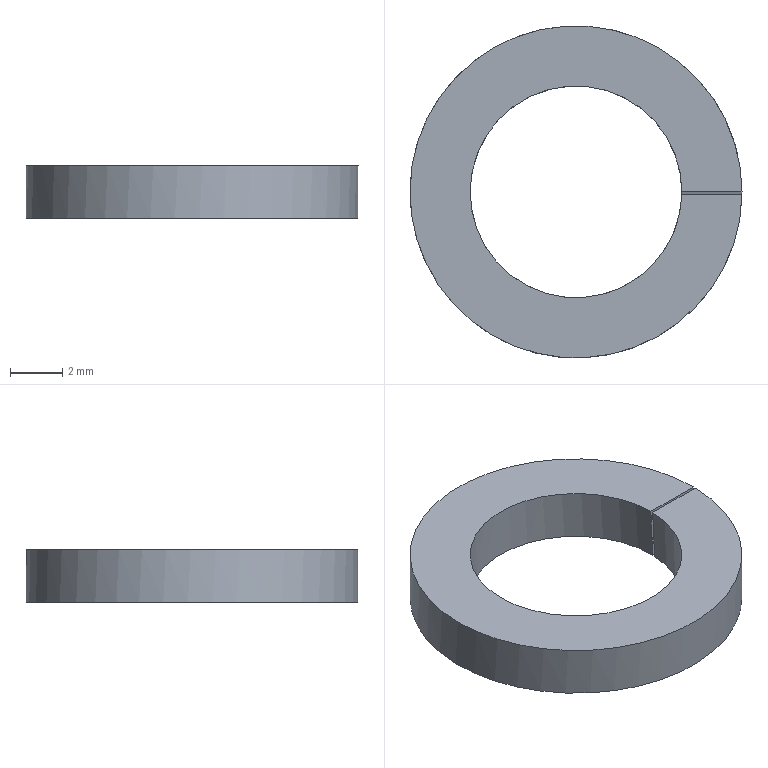Part | STEP file | SOLID | 1 solid | 6 faces | box 12.7 x 12.7 x 2 mm | volume 149.833 mm3 | plane 4 | cylinder 2 | commonest cylinder face diameters 8.1 x1 12.7 x1
STEP:
#1=CARTESIAN_POINT('',(0.,0.,0.));
#2=DIRECTION('',(0.,0.,1.));
#3=DIRECTION('',(1.,0.,0.));
#4=AXIS2_PLACEMENT_3D('',#1,#2,#3);
#5=CARTESIAN_POINT('',(6.349,-0.1,0.));
#6=VERTEX_POINT('',#5);
#7=CARTESIAN_POINT('',(6.347,-0.2048,-2.));
#8=VERTEX_POINT('',#7);
#9=CARTESIAN_POINT('',(0.,0.,1.908));
#10=DIRECTION('',(0.,0.9986,-0.05234));
#11=DIRECTION('',(0.,0.05234,0.9986));
#12=AXIS2_PLACEMENT_3D('',#9,#10,#11);
#13=ELLIPSE('',#12,121.331,6.35);
#14=CARTESIAN_POINT('',(0.,0.,-1.2));
#15=DIRECTION('',(0.,0.,1.));
#16=DIRECTION('',(1.,0.,0.));
#17=AXIS2_PLACEMENT_3D('',#14,#15,#16);
#18=CYLINDRICAL_SURFACE('',#17,6.35);
#19=CARTESIAN_POINT('',(6.267,1.2));
#20=CARTESIAN_POINT('',(6.267,1.17));
#21=CARTESIAN_POINT('',(6.267,1.109));
#22=CARTESIAN_POINT('',(6.266,1.018));
#23=CARTESIAN_POINT('',(6.265,0.9272));
#24=CARTESIAN_POINT('',(6.264,0.8363));
#25=CARTESIAN_POINT('',(6.264,0.7454));
#26=CARTESIAN_POINT('',(6.263,0.6545));
#27=CARTESIAN_POINT('',(6.262,0.5636));
#28=CARTESIAN_POINT('',(6.261,0.4726));
#29=CARTESIAN_POINT('',(6.261,0.3817));
#30=CARTESIAN_POINT('',(6.26,0.2908));
#31=CARTESIAN_POINT('',(6.259,0.1999));
#32=CARTESIAN_POINT('',(6.258,0.109));
#33=CARTESIAN_POINT('',(6.258,0.01808));
#34=CARTESIAN_POINT('',(6.257,-0.07282));
#35=CARTESIAN_POINT('',(6.256,-0.1637));
#36=CARTESIAN_POINT('',(6.255,-0.2546));
#37=CARTESIAN_POINT('',(6.255,-0.3455));
#38=CARTESIAN_POINT('',(6.254,-0.4364));
#39=CARTESIAN_POINT('',(6.253,-0.5273));
#40=CARTESIAN_POINT('',(6.252,-0.6182));
#41=CARTESIAN_POINT('',(6.252,-0.7091));
#42=CARTESIAN_POINT('',(6.251,-0.7697));
#43=CARTESIAN_POINT('',(6.251,-0.8));
#44=B_SPLINE_CURVE_WITH_KNOTS('',3,(#19,#20,#21,#22,#23,#24,#25,#26,#27,#28,#29,#30,#31,#32,#33,#34,#35,#36,#37,#38,#39,#40,#41,#42,#43),.UNSPECIFIED.,.F.,.F.,(4,1,1,1,1,1,1,1,1,1,1,1,1,1,1,1,1,1,1,1,1,1,4),(1.587,1.587,1.588,1.589,1.59,1.59,1.591,1.592,1.593,1.593,1.594,1.595,1.596,1.596,1.597,1.598,1.599,1.599,1.6,1.601,1.602,1.602,1.603),.QUASI_UNIFORM_KNOTS.);
#45=(GEOMETRIC_REPRESENTATION_CONTEXT(2)PARAMETRIC_REPRESENTATION_CONTEXT()REPRESENTATION_CONTEXT('',''));
#46=DEFINITIONAL_REPRESENTATION('',(#44),#45);
#47=PCURVE('',#18,#46);
#48=CARTESIAN_POINT('',(6.653,-0.1,0.));
#49=DIRECTION('',(0.,-0.9986,0.05234));
#50=DIRECTION('',(0.,-0.05234,-0.9986));
#51=AXIS2_PLACEMENT_3D('',#48,#49,#50);
#52=PLANE('',#51);
#53=CARTESIAN_POINT('',(-123.242,-6.653));
#54=CARTESIAN_POINT('',(-123.242,4.346));
#55=CARTESIAN_POINT('',(58.755,-1.153));
#56=CARTESIAN_POINT('',(240.752,-6.653));
#57=CARTESIAN_POINT('',(58.755,-12.152));
#58=CARTESIAN_POINT('',(-123.242,-17.651));
#59=CARTESIAN_POINT('',(-123.242,-6.653));
#60=(BOUNDED_CURVE()B_SPLINE_CURVE(2,(#53,#54,#55,#56,#57,#58,#59),.UNSPECIFIED.,.T.,.F.)B_SPLINE_CURVE_WITH_KNOTS((1,2,2,2,2,1),(-2.094,0.,2.094,4.189,6.283,8.378),.UNSPECIFIED.)CURVE()GEOMETRIC_REPRESENTATION_ITEM()RATIONAL_B_SPLINE_CURVE((1.,0.5,1.,0.5,1.,0.5,1.))REPRESENTATION_ITEM(''));
#61=(GEOMETRIC_REPRESENTATION_CONTEXT(2)PARAMETRIC_REPRESENTATION_CONTEXT()REPRESENTATION_CONTEXT('',''));
#62=DEFINITIONAL_REPRESENTATION('',(#60),#61);
#63=PCURVE('',#52,#62);
#64=SURFACE_CURVE('',#13,(#47,#63),.PCURVE_S1.);
#65=EDGE_CURVE('',#6,#8,#64,.T.);
#66=ORIENTED_EDGE('',*,*,#65,.F.);
#67=CARTESIAN_POINT('',(6.35,0.000137,-0.000003589));
#68=VERTEX_POINT('',#67);
#69=CARTESIAN_POINT('',(0.,0.,0.));
#70=DIRECTION('',(0.,0.,1.));
#71=DIRECTION('',(1.,0.,0.));
#72=AXIS2_PLACEMENT_3D('',#69,#70,#71);
#73=CIRCLE('',#72,6.35);
#74=CARTESIAN_POINT('',(0.,1.2));
#75=DIRECTION('',(1.,0.));
#76=VECTOR('',#75,1.);
#77=LINE('',#74,#76);
#78=(GEOMETRIC_REPRESENTATION_CONTEXT(2)PARAMETRIC_REPRESENTATION_CONTEXT()REPRESENTATION_CONTEXT('',''));
#79=DEFINITIONAL_REPRESENTATION('',(#77),#78);
#80=PCURVE('',#18,#79);
#81=CARTESIAN_POINT('',(0.,0.,0.));
#82=DIRECTION('',(0.,0.,1.));
#83=DIRECTION('',(1.,0.,0.));
#84=AXIS2_PLACEMENT_3D('',#81,#82,#83);
#85=PLANE('',#84);
#86=CARTESIAN_POINT('',(0.,0.));
#87=DIRECTION('',(1.,0.));
#88=AXIS2_PLACEMENT_2D('',#86,#87);
#89=CIRCLE('',#88,6.35);
#90=(GEOMETRIC_REPRESENTATION_CONTEXT(2)PARAMETRIC_REPRESENTATION_CONTEXT()REPRESENTATION_CONTEXT('',''));
#91=DEFINITIONAL_REPRESENTATION('',(#89),#90);
#92=PCURVE('',#85,#91);
#93=SURFACE_CURVE('',#73,(#80,#92),.PCURVE_S1.);
#94=EDGE_CURVE('',#68,#6,#93,.T.);
#95=ORIENTED_EDGE('',*,*,#94,.F.);
#96=CARTESIAN_POINT('',(6.349,-0.1047,-2.));
#97=VERTEX_POINT('',#96);
#98=CARTESIAN_POINT('',(0.,0.,-0.002619));
#99=DIRECTION('',(0.,0.9986,-0.05234));
#100=DIRECTION('',(0.,0.05234,0.9986));
#101=AXIS2_PLACEMENT_3D('',#98,#99,#100);
#102=ELLIPSE('',#101,121.331,6.35);
#103=CARTESIAN_POINT('',(0.00002158,1.2));
#104=CARTESIAN_POINT('',(-0.0002285,1.17));
#105=CARTESIAN_POINT('',(-0.0007287,1.109));
#106=CARTESIAN_POINT('',(-0.001479,1.018));
#107=CARTESIAN_POINT('',(-0.002229,0.9273));
#108=CARTESIAN_POINT('',(-0.00298,0.8363));
#109=CARTESIAN_POINT('',(-0.00373,0.7454));
#110=CARTESIAN_POINT('',(-0.00448,0.6545));
#111=CARTESIAN_POINT('',(-0.005231,0.5636));
#112=CARTESIAN_POINT('',(-0.005981,0.4727));
#113=CARTESIAN_POINT('',(-0.006731,0.3818));
#114=CARTESIAN_POINT('',(-0.007482,0.2909));
#115=CARTESIAN_POINT('',(-0.008232,0.2));
#116=CARTESIAN_POINT('',(-0.008982,0.1091));
#117=CARTESIAN_POINT('',(-0.009733,0.01814));
#118=CARTESIAN_POINT('',(-0.01048,-0.07276));
#119=CARTESIAN_POINT('',(-0.01123,-0.1637));
#120=CARTESIAN_POINT('',(-0.01198,-0.2546));
#121=CARTESIAN_POINT('',(-0.01273,-0.3455));
#122=CARTESIAN_POINT('',(-0.01348,-0.4364));
#123=CARTESIAN_POINT('',(-0.01423,-0.5273));
#124=CARTESIAN_POINT('',(-0.01498,-0.6182));
#125=CARTESIAN_POINT('',(-0.01574,-0.7091));
#126=CARTESIAN_POINT('',(-0.01624,-0.7697));
#127=CARTESIAN_POINT('',(-0.01649,-0.8));
#128=B_SPLINE_CURVE_WITH_KNOTS('',3,(#103,#104,#105,#106,#107,#108,#109,#110,#111,#112,#113,#114,#115,#116,#117,#118,#119,#120,#121,#122,#123,#124,#125,#126,#127),.UNSPECIFIED.,.F.,.F.,(4,1,1,1,1,1,1,1,1,1,1,1,1,1,1,1,1,1,1,1,1,1,4),(1.571,1.572,1.572,1.573,1.574,1.575,1.575,1.576,1.577,1.578,1.578,1.579,1.58,1.581,1.581,1.582,1.583,1.584,1.584,1.585,1.586,1.587,1.587),.QUASI_UNIFORM_KNOTS.);
#129=(GEOMETRIC_REPRESENTATION_CONTEXT(2)PARAMETRIC_REPRESENTATION_CONTEXT()REPRESENTATION_CONTEXT('',''));
#130=DEFINITIONAL_REPRESENTATION('',(#128),#129);
#131=PCURVE('',#18,#130);
#132=CARTESIAN_POINT('',(6.653,0.000137,-0.000003589));
#133=DIRECTION('',(0.,-0.9986,0.05234));
#134=DIRECTION('',(0.,-0.05234,-0.9986));
#135=AXIS2_PLACEMENT_3D('',#132,#133,#134);
#136=PLANE('',#135);
#137=CARTESIAN_POINT('',(-121.329,-6.653));
#138=CARTESIAN_POINT('',(-121.329,4.346));
#139=CARTESIAN_POINT('',(60.668,-1.153));
#140=CARTESIAN_POINT('',(242.666,-6.653));
#141=CARTESIAN_POINT('',(60.668,-12.152));
#142=CARTESIAN_POINT('',(-121.329,-17.651));
#143=CARTESIAN_POINT('',(-121.329,-6.653));
#144=(BOUNDED_CURVE()B_SPLINE_CURVE(2,(#137,#138,#139,#140,#141,#142,#143),.UNSPECIFIED.,.T.,.F.)B_SPLINE_CURVE_WITH_KNOTS((1,2,2,2,2,1),(-2.094,0.,2.094,4.189,6.283,8.378),.UNSPECIFIED.)CURVE()GEOMETRIC_REPRESENTATION_ITEM()RATIONAL_B_SPLINE_CURVE((1.,0.5,1.,0.5,1.,0.5,1.))REPRESENTATION_ITEM(''));
#145=(GEOMETRIC_REPRESENTATION_CONTEXT(2)PARAMETRIC_REPRESENTATION_CONTEXT()REPRESENTATION_CONTEXT('',''));
#146=DEFINITIONAL_REPRESENTATION('',(#144),#145);
#147=PCURVE('',#136,#146);
#148=SURFACE_CURVE('',#102,(#131,#147),.PCURVE_S1.);
#149=EDGE_CURVE('',#68,#97,#148,.T.);
#150=ORIENTED_EDGE('',*,*,#149,.T.);
#151=CARTESIAN_POINT('',(0.,0.,-2.));
#152=DIRECTION('',(0.,0.,1.));
#153=DIRECTION('',(1.,0.,0.));
#154=AXIS2_PLACEMENT_3D('',#151,#152,#153);
#155=CIRCLE('',#154,6.35);
#156=CARTESIAN_POINT('',(-6.283,-0.8));
#157=DIRECTION('',(1.,0.));
#158=VECTOR('',#157,1.);
#159=LINE('',#156,#158);
#160=(GEOMETRIC_REPRESENTATION_CONTEXT(2)PARAMETRIC_REPRESENTATION_CONTEXT()REPRESENTATION_CONTEXT('',''));
#161=DEFINITIONAL_REPRESENTATION('',(#159),#160);
#162=PCURVE('',#18,#161);
#163=CARTESIAN_POINT('',(0.,0.,-2.));
#164=DIRECTION('',(0.,0.,1.));
#165=DIRECTION('',(1.,0.,0.));
#166=AXIS2_PLACEMENT_3D('',#163,#164,#165);
#167=PLANE('',#166);
#168=CARTESIAN_POINT('',(0.,0.));
#169=DIRECTION('',(1.,0.));
#170=AXIS2_PLACEMENT_2D('',#168,#169);
#171=CIRCLE('',#170,6.35);
#172=(GEOMETRIC_REPRESENTATION_CONTEXT(2)PARAMETRIC_REPRESENTATION_CONTEXT()REPRESENTATION_CONTEXT('',''));
#173=DEFINITIONAL_REPRESENTATION('',(#171),#172);
#174=PCURVE('',#167,#173);
#175=SURFACE_CURVE('',#155,(#162,#174),.PCURVE_S1.);
#176=EDGE_CURVE('',#97,#8,#175,.T.);
#177=ORIENTED_EDGE('',*,*,#176,.T.);
#178=EDGE_LOOP('',(#66,#95,#150,#177));
#179=FACE_BOUND('',#178,.T.);
#180=ADVANCED_FACE('',(#179),#18,.T.);
#181=CARTESIAN_POINT('',(4.049,-0.1,0.));
#182=VERTEX_POINT('',#181);
#183=CARTESIAN_POINT('',(4.05,0.000137,-0.000003589));
#184=VERTEX_POINT('',#183);
#185=CARTESIAN_POINT('',(0.,0.,0.));
#186=DIRECTION('',(0.,0.,-1.));
#187=DIRECTION('',(1.,0.,0.));
#188=AXIS2_PLACEMENT_3D('',#185,#186,#187);
#189=CIRCLE('',#188,4.05);
#190=CARTESIAN_POINT('',(0.,0.,-1.2));
#191=DIRECTION('',(0.,0.,1.));
#192=DIRECTION('',(1.,0.,0.));
#193=AXIS2_PLACEMENT_3D('',#190,#191,#192);
#194=CYLINDRICAL_SURFACE('',#193,4.05);
#195=CARTESIAN_POINT('',(6.283,1.2));
#196=DIRECTION('',(-1.,0.));
#197=VECTOR('',#196,1.);
#198=LINE('',#195,#197);
#199=(GEOMETRIC_REPRESENTATION_CONTEXT(2)PARAMETRIC_REPRESENTATION_CONTEXT()REPRESENTATION_CONTEXT('',''));
#200=DEFINITIONAL_REPRESENTATION('',(#198),#199);
#201=PCURVE('',#194,#200);
#202=CARTESIAN_POINT('',(4.05,0.));
#203=CARTESIAN_POINT('',(4.05,-7.015));
#204=CARTESIAN_POINT('',(-2.025,-3.507));
#205=CARTESIAN_POINT('',(-8.1,0.));
#206=CARTESIAN_POINT('',(-2.025,3.507));
#207=CARTESIAN_POINT('',(4.05,7.015));
#208=CARTESIAN_POINT('',(4.05,0.));
#209=(BOUNDED_CURVE()B_SPLINE_CURVE(2,(#202,#203,#204,#205,#206,#207,#208),.UNSPECIFIED.,.T.,.F.)B_SPLINE_CURVE_WITH_KNOTS((1,2,2,2,2,1),(-2.094,0.,2.094,4.189,6.283,8.378),.UNSPECIFIED.)CURVE()GEOMETRIC_REPRESENTATION_ITEM()RATIONAL_B_SPLINE_CURVE((1.,0.5,1.,0.5,1.,0.5,1.))REPRESENTATION_ITEM(''));
#210=(GEOMETRIC_REPRESENTATION_CONTEXT(2)PARAMETRIC_REPRESENTATION_CONTEXT()REPRESENTATION_CONTEXT('',''));
#211=DEFINITIONAL_REPRESENTATION('',(#209),#210);
#212=PCURVE('',#85,#211);
#213=SURFACE_CURVE('',#189,(#201,#212),.PCURVE_S1.);
#214=EDGE_CURVE('',#182,#184,#213,.T.);
#215=ORIENTED_EDGE('',*,*,#214,.T.);
#216=CARTESIAN_POINT('',(4.049,-0.1047,-2.));
#217=VERTEX_POINT('',#216);
#218=CARTESIAN_POINT('',(0.,0.,-0.002619));
#219=DIRECTION('',(0.,-0.9986,0.05234));
#220=DIRECTION('',(0.,0.05234,0.9986));
#221=AXIS2_PLACEMENT_3D('',#218,#219,#220);
#222=ELLIPSE('',#221,77.385,4.05);
#223=CARTESIAN_POINT('',(-0.02585,-0.8));
#224=CARTESIAN_POINT('',(-0.02546,-0.7697));
#225=CARTESIAN_POINT('',(-0.02467,-0.7091));
#226=CARTESIAN_POINT('',(-0.0235,-0.6182));
#227=CARTESIAN_POINT('',(-0.02232,-0.5273));
#228=CARTESIAN_POINT('',(-0.02114,-0.4364));
#229=CARTESIAN_POINT('',(-0.01997,-0.3455));
#230=CARTESIAN_POINT('',(-0.01879,-0.2546));
#231=CARTESIAN_POINT('',(-0.01761,-0.1637));
#232=CARTESIAN_POINT('',(-0.01644,-0.07281));
#233=CARTESIAN_POINT('',(-0.01526,0.01809));
#234=CARTESIAN_POINT('',(-0.01408,0.109));
#235=CARTESIAN_POINT('',(-0.01291,0.1999));
#236=CARTESIAN_POINT('',(-0.01173,0.2908));
#237=CARTESIAN_POINT('',(-0.01055,0.3817));
#238=CARTESIAN_POINT('',(-0.009378,0.4727));
#239=CARTESIAN_POINT('',(-0.008202,0.5636));
#240=CARTESIAN_POINT('',(-0.007025,0.6545));
#241=CARTESIAN_POINT('',(-0.005849,0.7454));
#242=CARTESIAN_POINT('',(-0.004672,0.8363));
#243=CARTESIAN_POINT('',(-0.003496,0.9272));
#244=CARTESIAN_POINT('',(-0.002319,1.018));
#245=CARTESIAN_POINT('',(-0.001143,1.109));
#246=CARTESIAN_POINT('',(-0.0003583,1.17));
#247=CARTESIAN_POINT('',(0.00003384,1.2));
#248=B_SPLINE_CURVE_WITH_KNOTS('',3,(#223,#224,#225,#226,#227,#228,#229,#230,#231,#232,#233,#234,#235,#236,#237,#238,#239,#240,#241,#242,#243,#244,#245,#246,#247),.UNSPECIFIED.,.F.,.F.,(4,1,1,1,1,1,1,1,1,1,1,1,1,1,1,1,1,1,1,1,1,1,4),(4.687,4.688,4.689,4.69,4.691,4.692,4.694,4.695,4.696,4.697,4.698,4.699,4.701,4.702,4.703,4.704,4.705,4.707,4.708,4.709,4.71,4.711,4.712),.QUASI_UNIFORM_KNOTS.);
#249=(GEOMETRIC_REPRESENTATION_CONTEXT(2)PARAMETRIC_REPRESENTATION_CONTEXT()REPRESENTATION_CONTEXT('',''));
#250=DEFINITIONAL_REPRESENTATION('',(#248),#249);
#251=PCURVE('',#194,#250);
#252=CARTESIAN_POINT('',(0.002619,-6.653));
#253=DIRECTION('',(-1.,0.));
#254=AXIS2_PLACEMENT_2D('',#252,#253);
#255=ELLIPSE('',#254,77.385,4.05);
#256=(GEOMETRIC_REPRESENTATION_CONTEXT(2)PARAMETRIC_REPRESENTATION_CONTEXT()REPRESENTATION_CONTEXT('',''));
#257=DEFINITIONAL_REPRESENTATION('',(#255),#256);
#258=PCURVE('',#136,#257);
#259=SURFACE_CURVE('',#222,(#251,#258),.PCURVE_S1.);
#260=EDGE_CURVE('',#217,#184,#259,.T.);
#261=ORIENTED_EDGE('',*,*,#260,.F.);
#262=CARTESIAN_POINT('',(4.045,-0.2048,-2.));
#263=VERTEX_POINT('',#262);
#264=CARTESIAN_POINT('',(0.,0.,-2.));
#265=DIRECTION('',(0.,0.,-1.));
#266=DIRECTION('',(1.,0.,0.));
#267=AXIS2_PLACEMENT_3D('',#264,#265,#266);
#268=CIRCLE('',#267,4.05);
#269=CARTESIAN_POINT('',(6.283,-0.8));
#270=DIRECTION('',(-1.,0.));
#271=VECTOR('',#270,1.);
#272=LINE('',#269,#271);
#273=(GEOMETRIC_REPRESENTATION_CONTEXT(2)PARAMETRIC_REPRESENTATION_CONTEXT()REPRESENTATION_CONTEXT('',''));
#274=DEFINITIONAL_REPRESENTATION('',(#272),#273);
#275=PCURVE('',#194,#274);
#276=CARTESIAN_POINT('',(4.05,0.));
#277=CARTESIAN_POINT('',(4.05,-7.015));
#278=CARTESIAN_POINT('',(-2.025,-3.507));
#279=CARTESIAN_POINT('',(-8.1,0.));
#280=CARTESIAN_POINT('',(-2.025,3.507));
#281=CARTESIAN_POINT('',(4.05,7.015));
#282=CARTESIAN_POINT('',(4.05,0.));
#283=(BOUNDED_CURVE()B_SPLINE_CURVE(2,(#276,#277,#278,#279,#280,#281,#282),.UNSPECIFIED.,.T.,.F.)B_SPLINE_CURVE_WITH_KNOTS((1,2,2,2,2,1),(-2.094,0.,2.094,4.189,6.283,8.378),.UNSPECIFIED.)CURVE()GEOMETRIC_REPRESENTATION_ITEM()RATIONAL_B_SPLINE_CURVE((1.,0.5,1.,0.5,1.,0.5,1.))REPRESENTATION_ITEM(''));
#284=(GEOMETRIC_REPRESENTATION_CONTEXT(2)PARAMETRIC_REPRESENTATION_CONTEXT()REPRESENTATION_CONTEXT('',''));
#285=DEFINITIONAL_REPRESENTATION('',(#283),#284);
#286=PCURVE('',#167,#285);
#287=SURFACE_CURVE('',#268,(#275,#286),.PCURVE_S1.);
#288=EDGE_CURVE('',#263,#217,#287,.T.);
#289=ORIENTED_EDGE('',*,*,#288,.F.);
#290=CARTESIAN_POINT('',(0.,0.,1.908));
#291=DIRECTION('',(0.,-0.9986,0.05234));
#292=DIRECTION('',(0.,0.05234,0.9986));
#293=AXIS2_PLACEMENT_3D('',#290,#291,#292);
#294=ELLIPSE('',#293,77.385,4.05);
#295=CARTESIAN_POINT('',(6.233,-0.8));
#296=CARTESIAN_POINT('',(6.233,-0.7697));
#297=CARTESIAN_POINT('',(6.234,-0.7091));
#298=CARTESIAN_POINT('',(6.235,-0.6183));
#299=CARTESIAN_POINT('',(6.236,-0.5274));
#300=CARTESIAN_POINT('',(6.237,-0.4365));
#301=CARTESIAN_POINT('',(6.238,-0.3456));
#302=CARTESIAN_POINT('',(6.24,-0.2548));
#303=CARTESIAN_POINT('',(6.241,-0.1639));
#304=CARTESIAN_POINT('',(6.242,-0.07296));
#305=CARTESIAN_POINT('',(6.243,0.01794));
#306=CARTESIAN_POINT('',(6.244,0.1088));
#307=CARTESIAN_POINT('',(6.246,0.1998));
#308=CARTESIAN_POINT('',(6.247,0.2907));
#309=CARTESIAN_POINT('',(6.248,0.3816));
#310=CARTESIAN_POINT('',(6.249,0.4725));
#311=CARTESIAN_POINT('',(6.25,0.5634));
#312=CARTESIAN_POINT('',(6.251,0.6544));
#313=CARTESIAN_POINT('',(6.253,0.7453));
#314=CARTESIAN_POINT('',(6.254,0.8362));
#315=CARTESIAN_POINT('',(6.255,0.9272));
#316=CARTESIAN_POINT('',(6.256,1.018));
#317=CARTESIAN_POINT('',(6.257,1.109));
#318=CARTESIAN_POINT('',(6.258,1.17));
#319=CARTESIAN_POINT('',(6.258,1.2));
#320=B_SPLINE_CURVE_WITH_KNOTS('',3,(#295,#296,#297,#298,#299,#300,#301,#302,#303,#304,#305,#306,#307,#308,#309,#310,#311,#312,#313,#314,#315,#316,#317,#318,#319),.UNSPECIFIED.,.F.,.F.,(4,1,1,1,1,1,1,1,1,1,1,1,1,1,1,1,1,1,1,1,1,1,4),(4.662,4.663,4.664,4.665,4.667,4.668,4.669,4.67,4.671,4.672,4.674,4.675,4.676,4.677,4.678,4.679,4.681,4.682,4.683,4.684,4.685,4.687,4.688),.QUASI_UNIFORM_KNOTS.);
#321=(GEOMETRIC_REPRESENTATION_CONTEXT(2)PARAMETRIC_REPRESENTATION_CONTEXT()REPRESENTATION_CONTEXT('',''));
#322=DEFINITIONAL_REPRESENTATION('',(#320),#321);
#323=PCURVE('',#194,#322);
#324=CARTESIAN_POINT('',(-1.911,-6.653));
#325=DIRECTION('',(-1.,0.));
#326=AXIS2_PLACEMENT_2D('',#324,#325);
#327=ELLIPSE('',#326,77.385,4.05);
#328=(GEOMETRIC_REPRESENTATION_CONTEXT(2)PARAMETRIC_REPRESENTATION_CONTEXT()REPRESENTATION_CONTEXT('',''));
#329=DEFINITIONAL_REPRESENTATION('',(#327),#328);
#330=PCURVE('',#52,#329);
#331=SURFACE_CURVE('',#294,(#323,#330),.PCURVE_S1.);
#332=EDGE_CURVE('',#263,#182,#331,.T.);
#333=ORIENTED_EDGE('',*,*,#332,.T.);
#334=EDGE_LOOP('',(#215,#261,#289,#333));
#335=FACE_BOUND('',#334,.F.);
#336=ADVANCED_FACE('',(#335),#194,.F.);
#337=ORIENTED_EDGE('',*,*,#288,.F.);
#338=CARTESIAN_POINT('',(0.,-0.2048,-2.));
#339=DIRECTION('',(1.,0.,0.));
#340=VECTOR('',#339,1.);
#341=LINE('',#338,#340);
#342=CARTESIAN_POINT('',(0.,-0.2048));
#343=DIRECTION('',(1.,0.));
#344=VECTOR('',#343,1.);
#345=LINE('',#342,#344);
#346=(GEOMETRIC_REPRESENTATION_CONTEXT(2)PARAMETRIC_REPRESENTATION_CONTEXT()REPRESENTATION_CONTEXT('',''));
#347=DEFINITIONAL_REPRESENTATION('',(#345),#346);
#348=PCURVE('',#167,#347);
#349=CARTESIAN_POINT('',(2.003,-6.653));
#350=DIRECTION('',(0.,1.));
#351=VECTOR('',#350,1.);
#352=LINE('',#349,#351);
#353=(GEOMETRIC_REPRESENTATION_CONTEXT(2)PARAMETRIC_REPRESENTATION_CONTEXT()REPRESENTATION_CONTEXT('',''));
#354=DEFINITIONAL_REPRESENTATION('',(#352),#353);
#355=PCURVE('',#52,#354);
#356=SURFACE_CURVE('',#341,(#348,#355),.PCURVE_S1.);
#357=EDGE_CURVE('',#263,#8,#356,.T.);
#358=ORIENTED_EDGE('',*,*,#357,.T.);
#359=ORIENTED_EDGE('',*,*,#176,.F.);
#360=CARTESIAN_POINT('',(0.,-0.1047,-2.));
#361=DIRECTION('',(1.,0.,0.));
#362=VECTOR('',#361,1.);
#363=LINE('',#360,#362);
#364=CARTESIAN_POINT('',(0.,-0.1047));
#365=DIRECTION('',(1.,0.));
#366=VECTOR('',#365,1.);
#367=LINE('',#364,#366);
#368=(GEOMETRIC_REPRESENTATION_CONTEXT(2)PARAMETRIC_REPRESENTATION_CONTEXT()REPRESENTATION_CONTEXT('',''));
#369=DEFINITIONAL_REPRESENTATION('',(#367),#368);
#370=PCURVE('',#167,#369);
#371=CARTESIAN_POINT('',(2.003,-6.653));
#372=DIRECTION('',(0.,1.));
#373=VECTOR('',#372,1.);
#374=LINE('',#371,#373);
#375=(GEOMETRIC_REPRESENTATION_CONTEXT(2)PARAMETRIC_REPRESENTATION_CONTEXT()REPRESENTATION_CONTEXT('',''));
#376=DEFINITIONAL_REPRESENTATION('',(#374),#375);
#377=PCURVE('',#136,#376);
#378=SURFACE_CURVE('',#363,(#370,#377),.PCURVE_S1.);
#379=EDGE_CURVE('',#217,#97,#378,.T.);
#380=ORIENTED_EDGE('',*,*,#379,.F.);
#381=EDGE_LOOP('',(#337,#358,#359,#380));
#382=FACE_BOUND('',#381,.T.);
#383=ADVANCED_FACE('',(#382),#167,.F.);
#384=CARTESIAN_POINT('',(6.653,0.000137,-0.000003589));
#385=DIRECTION('',(-1.,0.,0.));
#386=VECTOR('',#385,1.);
#387=LINE('',#384,#386);
#388=CARTESIAN_POINT('',(6.653,0.000137));
#389=DIRECTION('',(-1.,0.));
#390=VECTOR('',#389,1.);
#391=LINE('',#388,#390);
#392=(GEOMETRIC_REPRESENTATION_CONTEXT(2)PARAMETRIC_REPRESENTATION_CONTEXT()REPRESENTATION_CONTEXT('',''));
#393=DEFINITIONAL_REPRESENTATION('',(#391),#392);
#394=PCURVE('',#85,#393);
#395=CARTESIAN_POINT('',(0.,0.));
#396=DIRECTION('',(0.,-1.));
#397=VECTOR('',#396,1.);
#398=LINE('',#395,#397);
#399=(GEOMETRIC_REPRESENTATION_CONTEXT(2)PARAMETRIC_REPRESENTATION_CONTEXT()REPRESENTATION_CONTEXT('',''));
#400=DEFINITIONAL_REPRESENTATION('',(#398),#399);
#401=PCURVE('',#136,#400);
#402=SURFACE_CURVE('',#387,(#394,#401),.PCURVE_S1.);
#403=EDGE_CURVE('',#68,#184,#402,.T.);
#404=ORIENTED_EDGE('',*,*,#403,.F.);
#405=ORIENTED_EDGE('',*,*,#94,.T.);
#406=CARTESIAN_POINT('',(6.653,-0.1,0.));
#407=DIRECTION('',(-1.,0.,0.));
#408=VECTOR('',#407,1.);
#409=LINE('',#406,#408);
#410=CARTESIAN_POINT('',(6.653,-0.1));
#411=DIRECTION('',(-1.,0.));
#412=VECTOR('',#411,1.);
#413=LINE('',#410,#412);
#414=(GEOMETRIC_REPRESENTATION_CONTEXT(2)PARAMETRIC_REPRESENTATION_CONTEXT()REPRESENTATION_CONTEXT('',''));
#415=DEFINITIONAL_REPRESENTATION('',(#413),#414);
#416=PCURVE('',#85,#415);
#417=CARTESIAN_POINT('',(0.,0.));
#418=DIRECTION('',(0.,-1.));
#419=VECTOR('',#418,1.);
#420=LINE('',#417,#419);
#421=(GEOMETRIC_REPRESENTATION_CONTEXT(2)PARAMETRIC_REPRESENTATION_CONTEXT()REPRESENTATION_CONTEXT('',''));
#422=DEFINITIONAL_REPRESENTATION('',(#420),#421);
#423=PCURVE('',#52,#422);
#424=SURFACE_CURVE('',#409,(#416,#423),.PCURVE_S1.);
#425=EDGE_CURVE('',#6,#182,#424,.T.);
#426=ORIENTED_EDGE('',*,*,#425,.T.);
#427=ORIENTED_EDGE('',*,*,#214,.T.);
#428=EDGE_LOOP('',(#404,#405,#426,#427));
#429=FACE_BOUND('',#428,.T.);
#430=ADVANCED_FACE('',(#429),#85,.T.);
#431=ORIENTED_EDGE('',*,*,#403,.T.);
#432=ORIENTED_EDGE('',*,*,#260,.F.);
#433=ORIENTED_EDGE('',*,*,#379,.T.);
#434=ORIENTED_EDGE('',*,*,#149,.F.);
#435=EDGE_LOOP('',(#431,#432,#433,#434));
#436=FACE_BOUND('',#435,.T.);
#437=ADVANCED_FACE('',(#436),#136,.T.);
#438=ORIENTED_EDGE('',*,*,#65,.T.);
#439=ORIENTED_EDGE('',*,*,#357,.F.);
#440=ORIENTED_EDGE('',*,*,#332,.T.);
#441=ORIENTED_EDGE('',*,*,#425,.F.);
#442=EDGE_LOOP('',(#438,#439,#440,#441));
#443=FACE_BOUND('',#442,.T.);
#444=ADVANCED_FACE('',(#443),#52,.F.);
#445=CLOSED_SHELL('',(#180,#336,#383,#430,#437,#444));
#446=MANIFOLD_SOLID_BREP('',#445);
#447=(LENGTH_UNIT()NAMED_UNIT(*)SI_UNIT(.MILLI.,.METRE.));
#448=UNCERTAINTY_MEASURE_WITH_UNIT(LENGTH_MEASURE(0.000001),#447,'','');
#449=(NAMED_UNIT(*)PLANE_ANGLE_UNIT()SI_UNIT($,.RADIAN.));
#450=(NAMED_UNIT(*)SI_UNIT($,.STERADIAN.)SOLID_ANGLE_UNIT());
#451=(GEOMETRIC_REPRESENTATION_CONTEXT(3)GLOBAL_UNCERTAINTY_ASSIGNED_CONTEXT((#448))GLOBAL_UNIT_ASSIGNED_CONTEXT((#447,#449,#450))REPRESENTATION_CONTEXT('',''));
#452=ADVANCED_BREP_SHAPE_REPRESENTATION('',(#4,#446),#451);